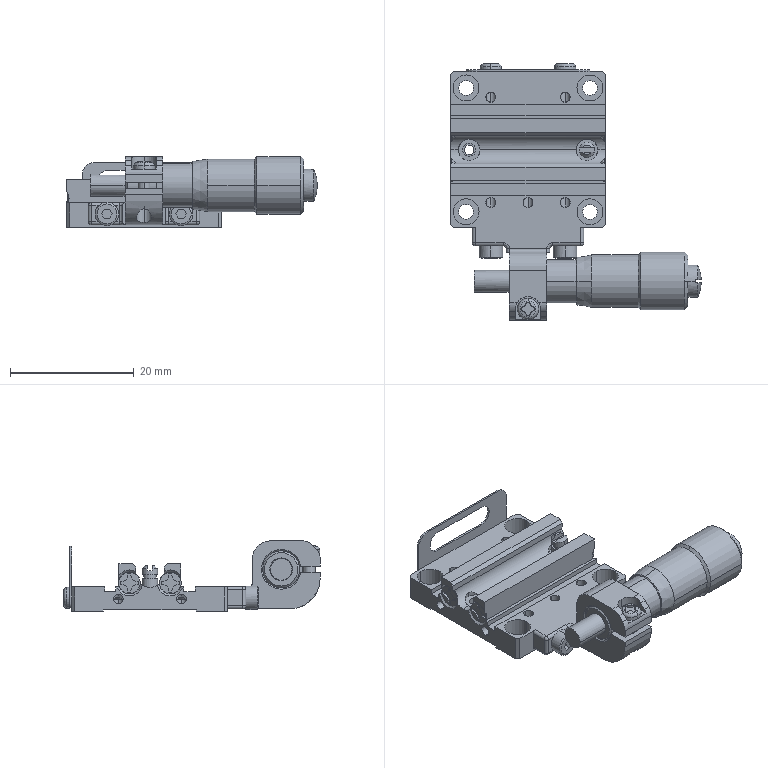Part | SolidWorks | features BaseBody 1 | 1 solid | 589 faces | box 40.495 x 41.4 x 11.45 mm | volume 4555 mm3 | plane 232 | cylinder 217 | cone 119 | torus 10 | sphere 7 | spline 4 | commonest cylinder face diameters 1.567 x32 2 x32 1.6 x30 2.4 x20 3.5 x20 1 x17